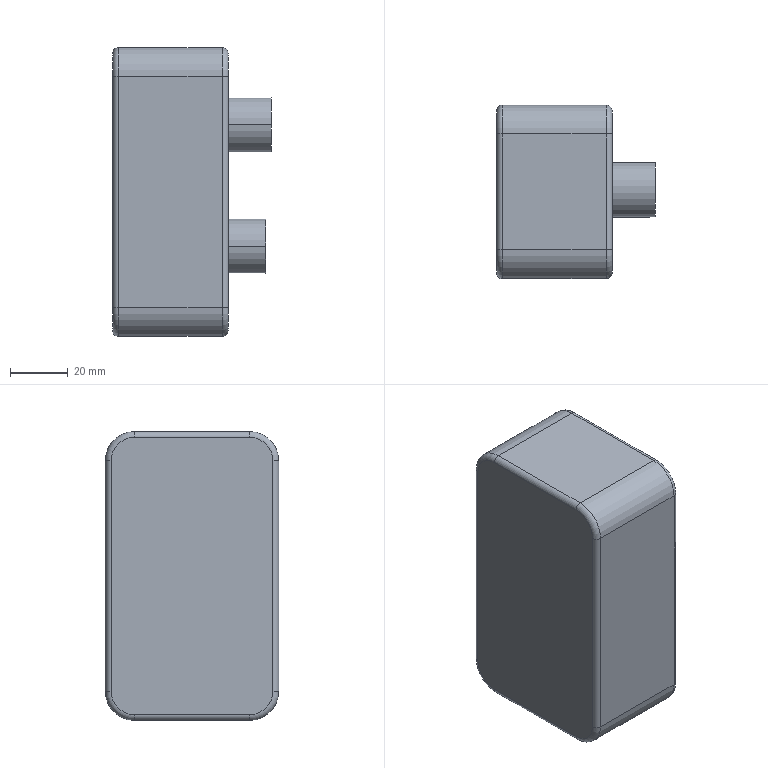Part | STEP file | PN_0013 | 1 solid | 32 faces | box 55 x 60 x 100 mm | volume 243898 mm3 | cylinder 16 | plane 8 | torus 8 | commonest cylinder face diameters 4 x8 18.89 x4 20 x4